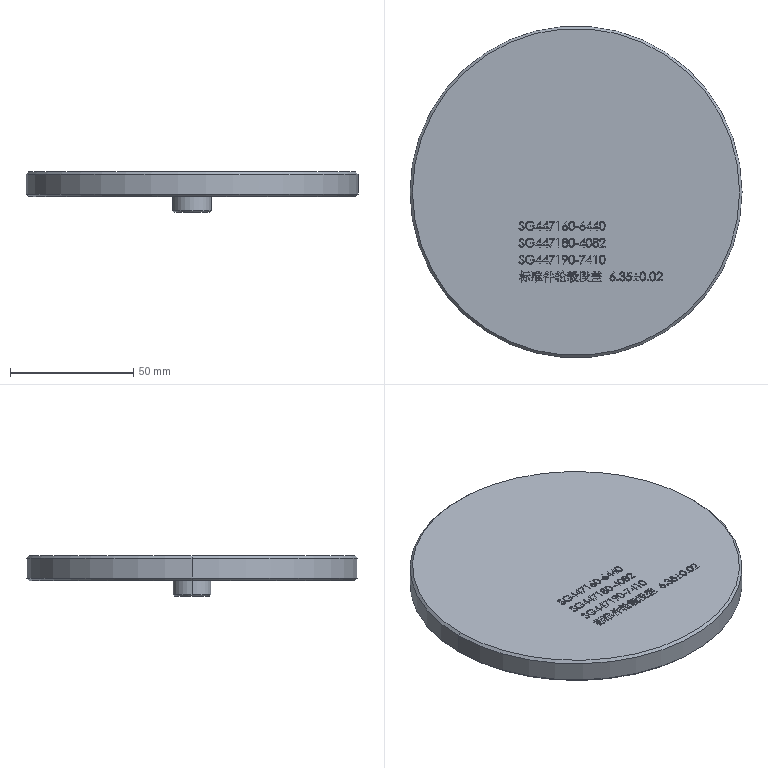Part | STEP file | PN_0001 hub standard part | 1 solid | 1057 faces | box 134.5 x 134.5 x 16.35 mm | volume 127475 mm3 | plane 676 | spline 367 | cone 8 | cylinder 6 | commonest cylinder face diameters 15.5 x2 100 x2 134.5 x2